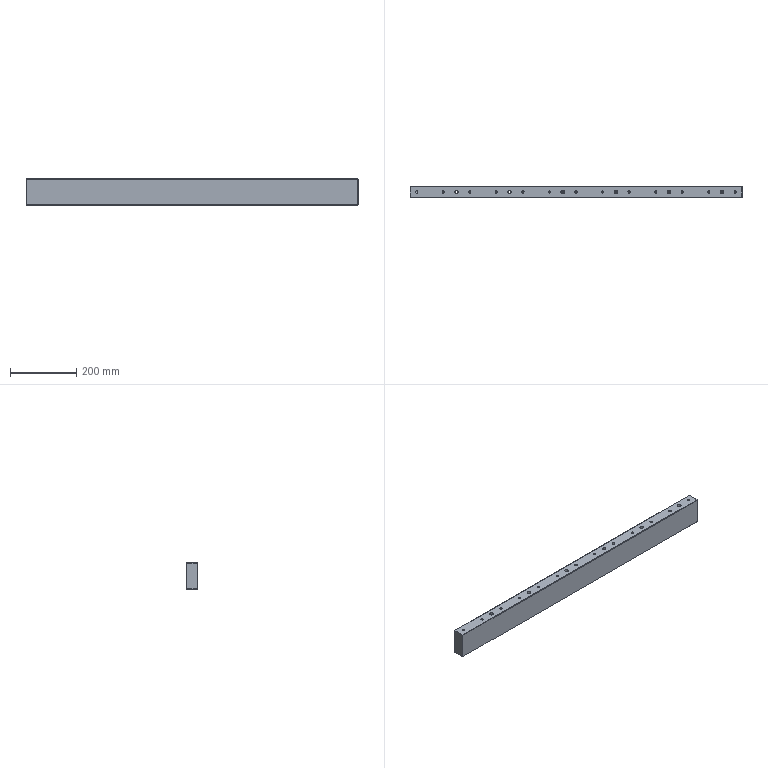Part | STEP file | TJ-DHQM-004-004 | 1 solid | 105 faces | box 1000 x 35 x 80 mm | volume 2758827 mm3 | cylinder 50 | plane 29 | cone 26 | commonest cylinder face diameters 6.8 x26 6.6 x12 11 x12